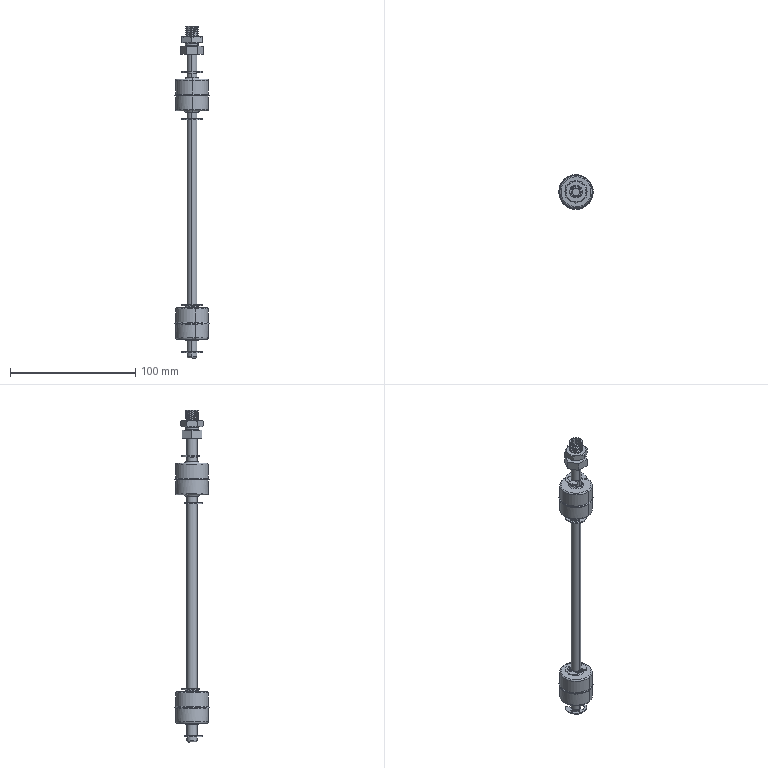Part | SolidWorks | 6 solids | 276 faces | box 27.5 x 27.5 x 265.5 mm | volume 30904 mm3 | cylinder 141 | plane 74 | torus 42 | cone 16 | spline 3 | commonest cylinder face diameters 10 x25 8.376 x22 1.829 x16 7.696 x12 8 x12 2.475 x8